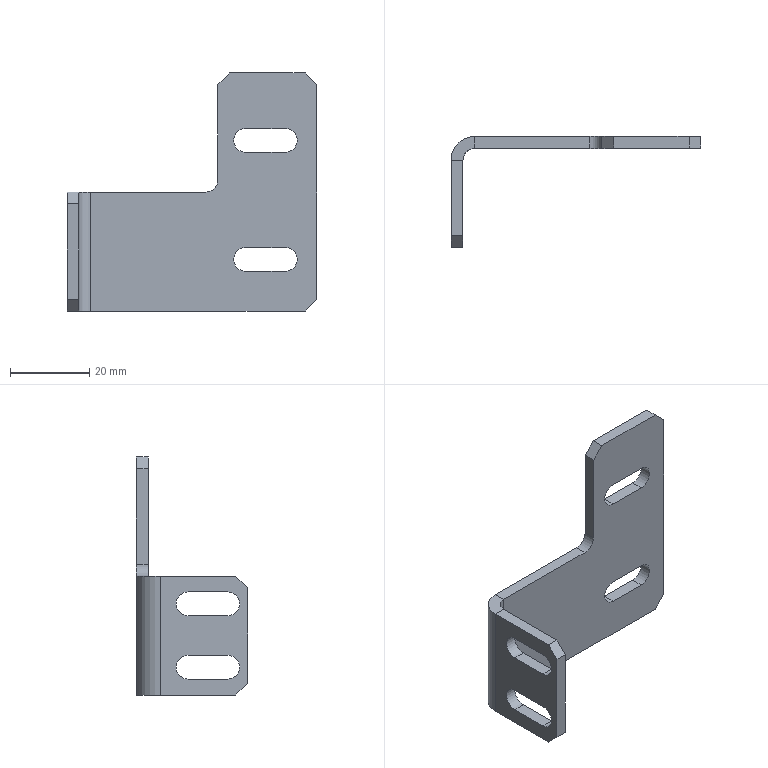Part | NX | features BREP 1 | 1 solid | 38 faces | box 63 x 28 x 60 mm | volume 8875 mm3 | plane 27 | cylinder 11 | commonest cylinder face diameters 6 x10 12 x1
STEP:
#1=CARTESIAN_POINT('',(0.,-3.,30.));
#2=VERTEX_POINT('',#1);
#3=CARTESIAN_POINT('',(-3.,-3.,30.));
#4=VERTEX_POINT('',#3);
#5=CARTESIAN_POINT('',(0.,-3.,30.));
#6=DIRECTION('',(-1.,0.,0.));
#7=VECTOR('',#6,1000.);
#8=LINE('',#5,#7);
#9=EDGE_CURVE('',#2,#4,#8,.T.);
#10=ORIENTED_EDGE('',*,*,#9,.F.);
#11=CARTESIAN_POINT('',(3.,0.,30.));
#12=VERTEX_POINT('',#11);
#13=CARTESIAN_POINT('',(3.,-3.,30.));
#14=DIRECTION('',(0.,0.,-1.));
#15=DIRECTION('',(1.,0.,0.));
#16=AXIS2_PLACEMENT_3D('',#13,#14,#15);
#17=CIRCLE('',#16,3.);
#18=EDGE_CURVE('',#2,#12,#17,.T.);
#19=ORIENTED_EDGE('',*,*,#18,.T.);
#20=CARTESIAN_POINT('',(3.,3.,30.));
#21=VERTEX_POINT('',#20);
#22=CARTESIAN_POINT('',(3.,3.,30.));
#23=DIRECTION('',(0.,-1.,0.));
#24=VECTOR('',#23,1000.);
#25=LINE('',#22,#24);
#26=EDGE_CURVE('',#21,#12,#25,.T.);
#27=ORIENTED_EDGE('',*,*,#26,.F.);
#28=CARTESIAN_POINT('',(3.,-3.,30.));
#29=DIRECTION('',(0.,0.,-1.));
#30=DIRECTION('',(1.,0.,0.));
#31=AXIS2_PLACEMENT_3D('',#28,#29,#30);
#32=CIRCLE('',#31,6.);
#33=EDGE_CURVE('',#4,#21,#32,.T.);
#34=ORIENTED_EDGE('',*,*,#33,.F.);
#35=EDGE_LOOP('',(#10,#19,#27,#34));
#36=FACE_BOUND('',#35,.T.);
#37=CARTESIAN_POINT('',(0.,-3.,30.));
#38=DIRECTION('',(0.,0.,1.));
#39=DIRECTION('',(-1.,0.,0.));
#40=AXIS2_PLACEMENT_3D('',#37,#38,#39);
#41=PLANE('',#40);
#42=ADVANCED_FACE('',(#36),#41,.T.);
#43=CARTESIAN_POINT('',(-3.,-22.,30.));
#44=VERTEX_POINT('',#43);
#45=CARTESIAN_POINT('',(-3.,-25.,30.));
#46=DIRECTION('',(0.,1.,0.));
#47=VECTOR('',#46,1000.);
#48=LINE('',#45,#47);
#49=EDGE_CURVE('',#44,#4,#48,.T.);
#50=ORIENTED_EDGE('',*,*,#49,.F.);
#51=CARTESIAN_POINT('',(0.,-22.,30.));
#52=VERTEX_POINT('',#51);
#53=CARTESIAN_POINT('',(3.,-22.,30.));
#54=DIRECTION('',(1.,0.,0.));
#55=VECTOR('',#54,1000.);
#56=LINE('',#53,#55);
#57=EDGE_CURVE('',#44,#52,#56,.T.);
#58=ORIENTED_EDGE('',*,*,#57,.T.);
#59=CARTESIAN_POINT('',(0.,-25.,30.));
#60=DIRECTION('',(0.,1.,0.));
#61=VECTOR('',#60,1000.);
#62=LINE('',#59,#61);
#63=EDGE_CURVE('',#52,#2,#62,.T.);
#64=ORIENTED_EDGE('',*,*,#63,.T.);
#65=ORIENTED_EDGE('',*,*,#9,.T.);
#66=EDGE_LOOP('',(#50,#58,#64,#65));
#67=FACE_BOUND('',#66,.T.);
#68=CARTESIAN_POINT('',(3.,3.,30.));
#69=DIRECTION('',(0.,0.,1.));
#70=DIRECTION('',(-1.,0.,0.));
#71=AXIS2_PLACEMENT_3D('',#68,#69,#70);
#72=PLANE('',#71);
#73=ADVANCED_FACE('',(#67),#72,.T.);
#74=CARTESIAN_POINT('',(3.,0.,0.));
#75=VERTEX_POINT('',#74);
#76=CARTESIAN_POINT('',(3.,3.,0.));
#77=VERTEX_POINT('',#76);
#78=CARTESIAN_POINT('',(3.,0.,0.));
#79=DIRECTION('',(0.,1.,0.));
#80=VECTOR('',#79,1000.);
#81=LINE('',#78,#80);
#82=EDGE_CURVE('',#75,#77,#81,.T.);
#83=ORIENTED_EDGE('',*,*,#82,.F.);
#84=CARTESIAN_POINT('',(0.,-3.,0.));
#85=VERTEX_POINT('',#84);
#86=CARTESIAN_POINT('',(3.,-3.,0.));
#87=DIRECTION('',(0.,0.,-1.));
#88=DIRECTION('',(1.,0.,0.));
#89=AXIS2_PLACEMENT_3D('',#86,#87,#88);
#90=CIRCLE('',#89,3.);
#91=EDGE_CURVE('',#85,#75,#90,.T.);
#92=ORIENTED_EDGE('',*,*,#91,.F.);
#93=CARTESIAN_POINT('',(-3.,-3.,0.));
#94=VERTEX_POINT('',#93);
#95=CARTESIAN_POINT('',(-3.,-3.,0.));
#96=DIRECTION('',(1.,0.,0.));
#97=VECTOR('',#96,1000.);
#98=LINE('',#95,#97);
#99=EDGE_CURVE('',#94,#85,#98,.T.);
#100=ORIENTED_EDGE('',*,*,#99,.F.);
#101=CARTESIAN_POINT('',(3.,-3.,0.));
#102=DIRECTION('',(0.,0.,-1.));
#103=DIRECTION('',(1.,0.,0.));
#104=AXIS2_PLACEMENT_3D('',#101,#102,#103);
#105=CIRCLE('',#104,6.);
#106=EDGE_CURVE('',#94,#77,#105,.T.);
#107=ORIENTED_EDGE('',*,*,#106,.T.);
#108=EDGE_LOOP('',(#83,#92,#100,#107));
#109=FACE_BOUND('',#108,.T.);
#110=CARTESIAN_POINT('',(3.,0.,0.));
#111=DIRECTION('',(0.,0.,-1.));
#112=DIRECTION('',(1.,0.,0.));
#113=AXIS2_PLACEMENT_3D('',#110,#111,#112);
#114=PLANE('',#113);
#115=ADVANCED_FACE('',(#109),#114,.T.);
#116=CARTESIAN_POINT('',(57.,3.,0.));
#117=VERTEX_POINT('',#116);
#118=CARTESIAN_POINT('',(0.,3.,0.));
#119=DIRECTION('',(1.,0.,0.));
#120=VECTOR('',#119,1000.);
#121=LINE('',#118,#120);
#122=EDGE_CURVE('',#77,#117,#121,.T.);
#123=ORIENTED_EDGE('',*,*,#122,.T.);
#124=CARTESIAN_POINT('',(57.,0.,0.));
#125=VERTEX_POINT('',#124);
#126=CARTESIAN_POINT('',(57.,-3.,0.));
#127=DIRECTION('',(0.,-1.,0.));
#128=VECTOR('',#127,1000.);
#129=LINE('',#126,#128);
#130=EDGE_CURVE('',#117,#125,#129,.T.);
#131=ORIENTED_EDGE('',*,*,#130,.T.);
#132=CARTESIAN_POINT('',(0.,0.,0.));
#133=DIRECTION('',(1.,0.,0.));
#134=VECTOR('',#133,1000.);
#135=LINE('',#132,#134);
#136=EDGE_CURVE('',#75,#125,#135,.T.);
#137=ORIENTED_EDGE('',*,*,#136,.F.);
#138=ORIENTED_EDGE('',*,*,#82,.T.);
#139=EDGE_LOOP('',(#123,#131,#137,#138));
#140=FACE_BOUND('',#139,.T.);
#141=CARTESIAN_POINT('',(-3.,-3.,0.));
#142=DIRECTION('',(0.,0.,-1.));
#143=DIRECTION('',(1.,0.,0.));
#144=AXIS2_PLACEMENT_3D('',#141,#142,#143);
#145=PLANE('',#144);
#146=ADVANCED_FACE('',(#140),#145,.T.);
#147=CARTESIAN_POINT('',(52.,0.,46.));
#148=VERTEX_POINT('',#147);
#149=CARTESIAN_POINT('',(42.,0.,46.));
#150=VERTEX_POINT('',#149);
#151=CARTESIAN_POINT('',(52.,0.,46.));
#152=DIRECTION('',(-1.,0.,0.));
#153=VECTOR('',#152,1000.);
#154=LINE('',#151,#153);
#155=EDGE_CURVE('',#148,#150,#154,.T.);
#156=ORIENTED_EDGE('',*,*,#155,.F.);
#157=CARTESIAN_POINT('',(52.,0.,40.));
#158=VERTEX_POINT('',#157);
#159=CARTESIAN_POINT('',(52.,0.,43.));
#160=DIRECTION('',(0.,-1.,0.));
#161=DIRECTION('',(0.,0.,1.));
#162=AXIS2_PLACEMENT_3D('',#159,#160,#161);
#163=CIRCLE('',#162,3.);
#164=EDGE_CURVE('',#158,#148,#163,.T.);
#165=ORIENTED_EDGE('',*,*,#164,.F.);
#166=CARTESIAN_POINT('',(42.,0.,40.));
#167=VERTEX_POINT('',#166);
#168=CARTESIAN_POINT('',(52.,0.,40.));
#169=DIRECTION('',(1.,0.,0.));
#170=VECTOR('',#169,1000.);
#171=LINE('',#168,#170);
#172=EDGE_CURVE('',#167,#158,#171,.T.);
#173=ORIENTED_EDGE('',*,*,#172,.F.);
#174=CARTESIAN_POINT('',(42.,0.,43.));
#175=DIRECTION('',(0.,-1.,0.));
#176=DIRECTION('',(0.,0.,1.));
#177=AXIS2_PLACEMENT_3D('',#174,#175,#176);
#178=CIRCLE('',#177,3.);
#179=EDGE_CURVE('',#150,#167,#178,.T.);
#180=ORIENTED_EDGE('',*,*,#179,.F.);
#181=EDGE_LOOP('',(#156,#165,#173,#180));
#182=FACE_BOUND('',#181,.T.);
#183=CARTESIAN_POINT('',(52.,0.,16.));
#184=VERTEX_POINT('',#183);
#185=CARTESIAN_POINT('',(42.,0.,16.));
#186=VERTEX_POINT('',#185);
#187=CARTESIAN_POINT('',(52.,0.,16.));
#188=DIRECTION('',(-1.,0.,0.));
#189=VECTOR('',#188,1000.);
#190=LINE('',#187,#189);
#191=EDGE_CURVE('',#184,#186,#190,.T.);
#192=ORIENTED_EDGE('',*,*,#191,.F.);
#193=CARTESIAN_POINT('',(52.,0.,10.));
#194=VERTEX_POINT('',#193);
#195=CARTESIAN_POINT('',(52.,0.,13.));
#196=DIRECTION('',(0.,-1.,0.));
#197=DIRECTION('',(0.,0.,1.));
#198=AXIS2_PLACEMENT_3D('',#195,#196,#197);
#199=CIRCLE('',#198,3.);
#200=EDGE_CURVE('',#194,#184,#199,.T.);
#201=ORIENTED_EDGE('',*,*,#200,.F.);
#202=CARTESIAN_POINT('',(42.,0.,10.));
#203=VERTEX_POINT('',#202);
#204=CARTESIAN_POINT('',(52.,0.,10.));
#205=DIRECTION('',(1.,0.,0.));
#206=VECTOR('',#205,1000.);
#207=LINE('',#204,#206);
#208=EDGE_CURVE('',#203,#194,#207,.T.);
#209=ORIENTED_EDGE('',*,*,#208,.F.);
#210=CARTESIAN_POINT('',(42.,0.,13.));
#211=DIRECTION('',(0.,-1.,0.));
#212=DIRECTION('',(0.,0.,1.));
#213=AXIS2_PLACEMENT_3D('',#210,#211,#212);
#214=CIRCLE('',#213,3.);
#215=EDGE_CURVE('',#186,#203,#214,.T.);
#216=ORIENTED_EDGE('',*,*,#215,.F.);
#217=EDGE_LOOP('',(#192,#201,#209,#216));
#218=FACE_BOUND('',#217,.T.);
#219=CARTESIAN_POINT('',(57.,0.,60.));
#220=VERTEX_POINT('',#219);
#221=CARTESIAN_POINT('',(38.,0.,60.));
#222=VERTEX_POINT('',#221);
#223=CARTESIAN_POINT('',(60.,0.,60.));
#224=DIRECTION('',(-1.,0.,0.));
#225=VECTOR('',#224,1000.);
#226=LINE('',#223,#225);
#227=EDGE_CURVE('',#220,#222,#226,.T.);
#228=ORIENTED_EDGE('',*,*,#227,.T.);
#229=CARTESIAN_POINT('',(35.,0.,57.));
#230=VERTEX_POINT('',#229);
#231=CARTESIAN_POINT('',(38.,0.,60.));
#232=DIRECTION('',(-0.7071,0.,-0.7071));
#233=VECTOR('',#232,1000.);
#234=LINE('',#231,#233);
#235=EDGE_CURVE('',#222,#230,#234,.T.);
#236=ORIENTED_EDGE('',*,*,#235,.T.);
#237=CARTESIAN_POINT('',(35.,0.,33.));
#238=VERTEX_POINT('',#237);
#239=CARTESIAN_POINT('',(35.,0.,30.));
#240=DIRECTION('',(0.,0.,-1.));
#241=VECTOR('',#240,1000.);
#242=LINE('',#239,#241);
#243=EDGE_CURVE('',#230,#238,#242,.T.);
#244=ORIENTED_EDGE('',*,*,#243,.T.);
#245=CARTESIAN_POINT('',(32.,0.,30.));
#246=VERTEX_POINT('',#245);
#247=CARTESIAN_POINT('',(32.,0.,33.));
#248=DIRECTION('',(0.,1.,0.));
#249=DIRECTION('',(0.,0.,1.));
#250=AXIS2_PLACEMENT_3D('',#247,#248,#249);
#251=CIRCLE('',#250,3.);
#252=EDGE_CURVE('',#238,#246,#251,.T.);
#253=ORIENTED_EDGE('',*,*,#252,.T.);
#254=CARTESIAN_POINT('',(0.,0.,30.));
#255=DIRECTION('',(1.,0.,0.));
#256=VECTOR('',#255,1000.);
#257=LINE('',#254,#256);
#258=EDGE_CURVE('',#12,#246,#257,.T.);
#259=ORIENTED_EDGE('',*,*,#258,.F.);
#260=CARTESIAN_POINT('',(3.,0.,30.));
#261=DIRECTION('',(0.,0.,-1.));
#262=VECTOR('',#261,1000.);
#263=LINE('',#260,#262);
#264=EDGE_CURVE('',#12,#75,#263,.T.);
#265=ORIENTED_EDGE('',*,*,#264,.T.);
#266=ORIENTED_EDGE('',*,*,#136,.T.);
#267=CARTESIAN_POINT('',(60.,0.,3.));
#268=VERTEX_POINT('',#267);
#269=CARTESIAN_POINT('',(57.,0.,0.));
#270=DIRECTION('',(0.7071,0.,0.7071));
#271=VECTOR('',#270,1000.);
#272=LINE('',#269,#271);
#273=EDGE_CURVE('',#125,#268,#272,.T.);
#274=ORIENTED_EDGE('',*,*,#273,.T.);
#275=CARTESIAN_POINT('',(60.,0.,57.));
#276=VERTEX_POINT('',#275);
#277=CARTESIAN_POINT('',(60.,0.,30.));
#278=DIRECTION('',(0.,0.,-1.));
#279=VECTOR('',#278,1000.);
#280=LINE('',#277,#279);
#281=EDGE_CURVE('',#276,#268,#280,.T.);
#282=ORIENTED_EDGE('',*,*,#281,.F.);
#283=CARTESIAN_POINT('',(60.,0.,57.));
#284=DIRECTION('',(-0.7071,0.,0.7071));
#285=VECTOR('',#284,1000.);
#286=LINE('',#283,#285);
#287=EDGE_CURVE('',#276,#220,#286,.T.);
#288=ORIENTED_EDGE('',*,*,#287,.T.);
#289=EDGE_LOOP('',(#228,#236,#244,#253,#259,#265,#266,#274,#282,#288));
#290=FACE_BOUND('',#289,.T.);
#291=CARTESIAN_POINT('',(0.,0.,30.));
#292=DIRECTION('',(0.,1.,0.));
#293=DIRECTION('',(0.,0.,-1.));
#294=AXIS2_PLACEMENT_3D('',#291,#292,#293);
#295=PLANE('',#294);
#296=ADVANCED_FACE('',(#182,#218,#290),#295,.F.);
#297=CARTESIAN_POINT('',(60.,3.,57.));
#298=VERTEX_POINT('',#297);
#299=CARTESIAN_POINT('',(60.,3.,3.));
#300=VERTEX_POINT('',#299);
#301=CARTESIAN_POINT('',(60.,3.,30.));
#302=DIRECTION('',(0.,0.,-1.));
#303=VECTOR('',#302,1000.);
#304=LINE('',#301,#303);
#305=EDGE_CURVE('',#298,#300,#304,.T.);
#306=ORIENTED_EDGE('',*,*,#305,.F.);
#307=CARTESIAN_POINT('',(60.,3.,57.));
#308=DIRECTION('',(0.,-1.,0.));
#309=VECTOR('',#308,1000.);
#310=LINE('',#307,#309);
#311=EDGE_CURVE('',#298,#276,#310,.T.);
#312=ORIENTED_EDGE('',*,*,#311,.T.);
#313=ORIENTED_EDGE('',*,*,#281,.T.);
#314=CARTESIAN_POINT('',(60.,3.,3.));
#315=DIRECTION('',(0.,1.,0.));
#316=VECTOR('',#315,1000.);
#317=LINE('',#314,#316);
#318=EDGE_CURVE('',#268,#300,#317,.T.);
#319=ORIENTED_EDGE('',*,*,#318,.T.);
#320=EDGE_LOOP('',(#306,#312,#313,#319));
#321=FACE_BOUND('',#320,.T.);
#322=CARTESIAN_POINT('',(60.,3.,30.));
#323=DIRECTION('',(1.,0.,0.));
#324=DIRECTION('',(0.,0.,1.));
#325=AXIS2_PLACEMENT_3D('',#322,#323,#324);
#326=PLANE('',#325);
#327=ADVANCED_FACE('',(#321),#326,.T.);
#328=CARTESIAN_POINT('',(52.,3.,46.));
#329=VERTEX_POINT('',#328);
#330=CARTESIAN_POINT('',(52.,3.,40.));
#331=VERTEX_POINT('',#330);
#332=CARTESIAN_POINT('',(52.,3.,43.));
#333=DIRECTION('',(0.,1.,0.));
#334=DIRECTION('',(0.,0.,1.));
#335=AXIS2_PLACEMENT_3D('',#332,#333,#334);
#336=CIRCLE('',#335,3.);
#337=EDGE_CURVE('',#329,#331,#336,.T.);
#338=ORIENTED_EDGE('',*,*,#337,.F.);
#339=CARTESIAN_POINT('',(42.,3.,46.));
#340=VERTEX_POINT('',#339);
#341=CARTESIAN_POINT('',(52.,3.,46.));
#342=DIRECTION('',(1.,0.,0.));
#343=VECTOR('',#342,1000.);
#344=LINE('',#341,#343);
#345=EDGE_CURVE('',#340,#329,#344,.T.);
#346=ORIENTED_EDGE('',*,*,#345,.F.);
#347=CARTESIAN_POINT('',(42.,3.,40.));
#348=VERTEX_POINT('',#347);
#349=CARTESIAN_POINT('',(42.,3.,43.));
#350=DIRECTION('',(0.,1.,0.));
#351=DIRECTION('',(0.,0.,1.));
#352=AXIS2_PLACEMENT_3D('',#349,#350,#351);
#353=CIRCLE('',#352,3.);
#354=EDGE_CURVE('',#348,#340,#353,.T.);
#355=ORIENTED_EDGE('',*,*,#354,.F.);
#356=CARTESIAN_POINT('',(52.,3.,40.));
#357=DIRECTION('',(-1.,0.,0.));
#358=VECTOR('',#357,1000.);
#359=LINE('',#356,#358);
#360=EDGE_CURVE('',#331,#348,#359,.T.);
#361=ORIENTED_EDGE('',*,*,#360,.F.);
#362=EDGE_LOOP('',(#338,#346,#355,#361));
#363=FACE_BOUND('',#362,.T.);
#364=CARTESIAN_POINT('',(52.,3.,16.));
#365=VERTEX_POINT('',#364);
#366=CARTESIAN_POINT('',(52.,3.,10.));
#367=VERTEX_POINT('',#366);
#368=CARTESIAN_POINT('',(52.,3.,13.));
#369=DIRECTION('',(0.,1.,0.));
#370=DIRECTION('',(0.,0.,1.));
#371=AXIS2_PLACEMENT_3D('',#368,#369,#370);
#372=CIRCLE('',#371,3.);
#373=EDGE_CURVE('',#365,#367,#372,.T.);
#374=ORIENTED_EDGE('',*,*,#373,.F.);
#375=CARTESIAN_POINT('',(42.,3.,16.));
#376=VERTEX_POINT('',#375);
#377=CARTESIAN_POINT('',(52.,3.,16.));
#378=DIRECTION('',(1.,0.,0.));
#379=VECTOR('',#378,1000.);
#380=LINE('',#377,#379);
#381=EDGE_CURVE('',#376,#365,#380,.T.);
#382=ORIENTED_EDGE('',*,*,#381,.F.);
#383=CARTESIAN_POINT('',(42.,3.,10.));
#384=VERTEX_POINT('',#383);
#385=CARTESIAN_POINT('',(42.,3.,13.));
#386=DIRECTION('',(0.,1.,0.));
#387=DIRECTION('',(0.,0.,1.));
#388=AXIS2_PLACEMENT_3D('',#385,#386,#387);
#389=CIRCLE('',#388,3.);
#390=EDGE_CURVE('',#384,#376,#389,.T.);
#391=ORIENTED_EDGE('',*,*,#390,.F.);
#392=CARTESIAN_POINT('',(52.,3.,10.));
#393=DIRECTION('',(-1.,0.,0.));
#394=VECTOR('',#393,1000.);
#395=LINE('',#392,#394);
#396=EDGE_CURVE('',#367,#384,#395,.T.);
#397=ORIENTED_EDGE('',*,*,#396,.F.);
#398=EDGE_LOOP('',(#374,#382,#391,#397));
#399=FACE_BOUND('',#398,.T.);
#400=CARTESIAN_POINT('',(35.,3.,57.));
#401=VERTEX_POINT('',#400);
#402=CARTESIAN_POINT('',(35.,3.,33.));
#403=VERTEX_POINT('',#402);
#404=CARTESIAN_POINT('',(35.,3.,30.));
#405=DIRECTION('',(0.,0.,-1.));
#406=VECTOR('',#405,1000.);
#407=LINE('',#404,#406);
#408=EDGE_CURVE('',#401,#403,#407,.T.);
#409=ORIENTED_EDGE('',*,*,#408,.F.);
#410=CARTESIAN_POINT('',(38.,3.,60.));
#411=VERTEX_POINT('',#410);
#412=CARTESIAN_POINT('',(4.,3.,26.));
#413=DIRECTION('',(0.7071,0.,0.7071));
#414=VECTOR('',#413,1000.);
#415=LINE('',#412,#414);
#416=EDGE_CURVE('',#401,#411,#415,.T.);
#417=ORIENTED_EDGE('',*,*,#416,.T.);
#418=CARTESIAN_POINT('',(57.,3.,60.));
#419=VERTEX_POINT('',#418);
#420=CARTESIAN_POINT('',(60.,3.,60.));
#421=DIRECTION('',(-1.,0.,0.));
#422=VECTOR('',#421,1000.);
#423=LINE('',#420,#422);
#424=EDGE_CURVE('',#419,#411,#423,.T.);
#425=ORIENTED_EDGE('',*,*,#424,.F.);
#426=CARTESIAN_POINT('',(43.5,3.,73.5));
#427=DIRECTION('',(0.7071,0.,-0.7071));
#428=VECTOR('',#427,1000.);
#429=LINE('',#426,#428);
#430=EDGE_CURVE('',#419,#298,#429,.T.);
#431=ORIENTED_EDGE('',*,*,#430,.T.);
#432=ORIENTED_EDGE('',*,*,#305,.T.);
#433=CARTESIAN_POINT('',(43.5,3.,-13.5));
#434=DIRECTION('',(-0.7071,0.,-0.7071));
#435=VECTOR('',#434,1000.);
#436=LINE('',#433,#435);
#437=EDGE_CURVE('',#300,#117,#436,.T.);
#438=ORIENTED_EDGE('',*,*,#437,.T.);
#439=ORIENTED_EDGE('',*,*,#122,.F.);
#440=CARTESIAN_POINT('',(3.,3.,30.));
#441=DIRECTION('',(0.,0.,-1.));
#442=VECTOR('',#441,1000.);
#443=LINE('',#440,#442);
#444=EDGE_CURVE('',#21,#77,#443,.T.);
#445=ORIENTED_EDGE('',*,*,#444,.F.);
#446=CARTESIAN_POINT('',(32.,3.,30.));
#447=VERTEX_POINT('',#446);
#448=CARTESIAN_POINT('',(0.,3.,30.));
#449=DIRECTION('',(1.,0.,0.));
#450=VECTOR('',#449,1000.);
#451=LINE('',#448,#450);
#452=EDGE_CURVE('',#21,#447,#451,.T.);
#453=ORIENTED_EDGE('',*,*,#452,.T.);
#454=CARTESIAN_POINT('',(32.,3.,33.));
#455=DIRECTION('',(0.,-1.,0.));
#456=DIRECTION('',(0.,0.,1.));
#457=AXIS2_PLACEMENT_3D('',#454,#455,#456);
#458=CIRCLE('',#457,3.);
#459=EDGE_CURVE('',#447,#403,#458,.T.);
#460=ORIENTED_EDGE('',*,*,#459,.T.);
#461=EDGE_LOOP('',(#409,#417,#425,#431,#432,#438,#439,#445,#453,#460));
#462=FACE_BOUND('',#461,.T.);
#463=CARTESIAN_POINT('',(0.,3.,30.));
#464=DIRECTION('',(0.,1.,0.));
#465=DIRECTION('',(0.,0.,-1.));
#466=AXIS2_PLACEMENT_3D('',#463,#464,#465);
#467=PLANE('',#466);
#468=ADVANCED_FACE('',(#363,#399,#462),#467,.T.);
#469=ORIENTED_EDGE('',*,*,#106,.F.);
#470=CARTESIAN_POINT('',(-3.,-3.,30.));
#471=DIRECTION('',(0.,0.,-1.));
#472=VECTOR('',#471,1000.);
#473=LINE('',#470,#472);
#474=EDGE_CURVE('',#4,#94,#473,.T.);
#475=ORIENTED_EDGE('',*,*,#474,.F.);
#476=ORIENTED_EDGE('',*,*,#33,.T.);
#477=ORIENTED_EDGE('',*,*,#444,.T.);
#478=EDGE_LOOP('',(#469,#475,#476,#477));
#479=FACE_BOUND('',#478,.T.);
#480=CARTESIAN_POINT('',(3.,-3.,30.));
#481=DIRECTION('',(0.,0.,-1.));
#482=DIRECTION('',(1.,0.,0.));
#483=AXIS2_PLACEMENT_3D('',#480,#481,#482);
#484=CYLINDRICAL_SURFACE('',#483,6.);
#485=ADVANCED_FACE('',(#479),#484,.T.);
#486=CARTESIAN_POINT('',(-3.,-10.,26.));
#487=VERTEX_POINT('',#486);
#488=CARTESIAN_POINT('',(-3.,-20.,26.));
#489=VERTEX_POINT('',#488);
#490=CARTESIAN_POINT('',(-3.,-10.,26.));
#491=DIRECTION('',(0.,-1.,0.));
#492=VECTOR('',#491,1000.);
#493=LINE('',#490,#492);
#494=EDGE_CURVE('',#487,#489,#493,.T.);
#495=ORIENTED_EDGE('',*,*,#494,.T.);
#496=CARTESIAN_POINT('',(-3.,-20.,20.));
#497=VERTEX_POINT('',#496);
#498=CARTESIAN_POINT('',(-3.,-20.,23.));
#499=DIRECTION('',(1.,0.,0.));
#500=DIRECTION('',(0.,0.,1.));
#501=AXIS2_PLACEMENT_3D('',#498,#499,#500);
#502=CIRCLE('',#501,3.);
#503=EDGE_CURVE('',#489,#497,#502,.T.);
#504=ORIENTED_EDGE('',*,*,#503,.T.);
#505=CARTESIAN_POINT('',(-3.,-10.,20.));
#506=VERTEX_POINT('',#505);
#507=CARTESIAN_POINT('',(-3.,-10.,20.));
#508=DIRECTION('',(0.,1.,0.));
#509=VECTOR('',#508,1000.);
#510=LINE('',#507,#509);
#511=EDGE_CURVE('',#497,#506,#510,.T.);
#512=ORIENTED_EDGE('',*,*,#511,.T.);
#513=CARTESIAN_POINT('',(-3.,-10.,23.));
#514=DIRECTION('',(1.,0.,0.));
#515=DIRECTION('',(0.,0.,1.));
#516=AXIS2_PLACEMENT_3D('',#513,#514,#515);
#517=CIRCLE('',#516,3.);
#518=EDGE_CURVE('',#506,#487,#517,.T.);
#519=ORIENTED_EDGE('',*,*,#518,.T.);
#520=EDGE_LOOP('',(#495,#504,#512,#519));
#521=FACE_BOUND('',#520,.T.);
#522=CARTESIAN_POINT('',(-3.,-10.,10.));
#523=VERTEX_POINT('',#522);
#524=CARTESIAN_POINT('',(-3.,-20.,10.));
#525=VERTEX_POINT('',#524);
#526=CARTESIAN_POINT('',(-3.,-10.,10.));
#527=DIRECTION('',(0.,-1.,0.));
#528=VECTOR('',#527,1000.);
#529=LINE('',#526,#528);
#530=EDGE_CURVE('',#523,#525,#529,.T.);
#531=ORIENTED_EDGE('',*,*,#530,.T.);
#532=CARTESIAN_POINT('',(-3.,-20.,4.));
#533=VERTEX_POINT('',#532);
#534=CARTESIAN_POINT('',(-3.,-20.,7.));
#535=DIRECTION('',(1.,0.,0.));
#536=DIRECTION('',(0.,0.,1.));
#537=AXIS2_PLACEMENT_3D('',#534,#535,#536);
#538=CIRCLE('',#537,3.);
#539=EDGE_CURVE('',#525,#533,#538,.T.);
#540=ORIENTED_EDGE('',*,*,#539,.T.);
#541=CARTESIAN_POINT('',(-3.,-10.,4.));
#542=VERTEX_POINT('',#541);
#543=CARTESIAN_POINT('',(-3.,-10.,4.));
#544=DIRECTION('',(0.,1.,0.));
#545=VECTOR('',#544,1000.);
#546=LINE('',#543,#545);
#547=EDGE_CURVE('',#533,#542,#546,.T.);
#548=ORIENTED_EDGE('',*,*,#547,.T.);
#549=CARTESIAN_POINT('',(-3.,-10.,7.));
#550=DIRECTION('',(1.,0.,0.));
#551=DIRECTION('',(0.,0.,1.));
#552=AXIS2_PLACEMENT_3D('',#549,#550,#551);
#553=CIRCLE('',#552,3.);
#554=EDGE_CURVE('',#542,#523,#553,.T.);
#555=ORIENTED_EDGE('',*,*,#554,.T.);
#556=EDGE_LOOP('',(#531,#540,#548,#555));
#557=FACE_BOUND('',#556,.T.);
#558=CARTESIAN_POINT('',(-3.,-25.,27.));
#559=VERTEX_POINT('',#558);
#560=CARTESIAN_POINT('',(-3.,-25.,3.));
#561=VERTEX_POINT('',#560);
#562=CARTESIAN_POINT('',(-3.,-25.,30.));
#563=DIRECTION('',(0.,0.,-1.));
#564=VECTOR('',#563,1000.);
#565=LINE('',#562,#564);
#566=EDGE_CURVE('',#559,#561,#565,.T.);
#567=ORIENTED_EDGE('',*,*,#566,.F.);
#568=CARTESIAN_POINT('',(-3.,-23.5,28.5));
#569=DIRECTION('',(0.,0.7071,0.7071));
#570=VECTOR('',#569,1000.);
#571=LINE('',#568,#570);
#572=EDGE_CURVE('',#559,#44,#571,.T.);
#573=ORIENTED_EDGE('',*,*,#572,.T.);
#574=ORIENTED_EDGE('',*,*,#49,.T.);
#575=ORIENTED_EDGE('',*,*,#474,.T.);
#576=CARTESIAN_POINT('',(-3.,-22.,0.));
#577=VERTEX_POINT('',#576);
#578=CARTESIAN_POINT('',(-3.,-25.,0.));
#579=DIRECTION('',(0.,1.,0.));
#580=VECTOR('',#579,1000.);
#581=LINE('',#578,#580);
#582=EDGE_CURVE('',#577,#94,#581,.T.);
#583=ORIENTED_EDGE('',*,*,#582,.F.);
#584=CARTESIAN_POINT('',(-3.,-38.5,16.5));
#585=DIRECTION('',(0.,-0.7071,0.7071));
#586=VECTOR('',#585,1000.);
#587=LINE('',#584,#586);
#588=EDGE_CURVE('',#577,#561,#587,.T.);
#589=ORIENTED_EDGE('',*,*,#588,.T.);
#590=EDGE_LOOP('',(#567,#573,#574,#575,#583,#589));
#591=FACE_BOUND('',#590,.T.);
#592=CARTESIAN_POINT('',(-3.,-25.,30.));
#593=DIRECTION('',(-1.,0.,0.));
#594=DIRECTION('',(0.,0.,-1.));
#595=AXIS2_PLACEMENT_3D('',#592,#593,#594);
#596=PLANE('',#595);
#597=ADVANCED_FACE('',(#521,#557,#591),#596,.T.);
#598=CARTESIAN_POINT('',(0.,-25.,27.));
#599=VERTEX_POINT('',#598);
#600=CARTESIAN_POINT('',(0.,-25.,3.));
#601=VERTEX_POINT('',#600);
#602=CARTESIAN_POINT('',(0.,-25.,30.));
#603=DIRECTION('',(0.,0.,-1.));
#604=VECTOR('',#603,1000.);
#605=LINE('',#602,#604);
#606=EDGE_CURVE('',#599,#601,#605,.T.);
#607=ORIENTED_EDGE('',*,*,#606,.F.);
#608=CARTESIAN_POINT('',(0.,-25.,27.));
#609=DIRECTION('',(-1.,0.,0.));
#610=VECTOR('',#609,1000.);
#611=LINE('',#608,#610);
#612=EDGE_CURVE('',#599,#559,#611,.T.);
#613=ORIENTED_EDGE('',*,*,#612,.T.);
#614=ORIENTED_EDGE('',*,*,#566,.T.);
#615=CARTESIAN_POINT('',(0.,-25.,3.));
#616=DIRECTION('',(1.,0.,0.));
#617=VECTOR('',#616,1000.);
#618=LINE('',#615,#617);
#619=EDGE_CURVE('',#561,#601,#618,.T.);
#620=ORIENTED_EDGE('',*,*,#619,.T.);
#621=EDGE_LOOP('',(#607,#613,#614,#620));
#622=FACE_BOUND('',#621,.T.);
#623=CARTESIAN_POINT('',(0.,-25.,30.));
#624=DIRECTION('',(0.,-1.,0.));
#625=DIRECTION('',(0.,0.,1.));
#626=AXIS2_PLACEMENT_3D('',#623,#624,#625);
#627=PLANE('',#626);
#628=ADVANCED_FACE('',(#622),#627,.T.);
#629=CARTESIAN_POINT('',(0.,-20.,26.));
#630=VERTEX_POINT('',#629);
#631=CARTESIAN_POINT('',(0.,-20.,20.));
#632=VERTEX_POINT('',#631);
#633=CARTESIAN_POINT('',(0.,-20.,23.));
#634=DIRECTION('',(1.,0.,0.));
#635=DIRECTION('',(0.,0.,-1.));
#636=AXIS2_PLACEMENT_3D('',#633,#634,#635);
#637=CIRCLE('',#636,3.);
#638=EDGE_CURVE('',#630,#632,#637,.T.);
#639=ORIENTED_EDGE('',*,*,#638,.F.);
#640=CARTESIAN_POINT('',(0.,-10.,26.));
#641=VERTEX_POINT('',#640);
#642=CARTESIAN_POINT('',(0.,-10.,26.));
#643=DIRECTION('',(0.,-1.,0.));
#644=VECTOR('',#643,1000.);
#645=LINE('',#642,#644);
#646=EDGE_CURVE('',#641,#630,#645,.T.);
#647=ORIENTED_EDGE('',*,*,#646,.F.);
#648=CARTESIAN_POINT('',(0.,-10.,20.));
#649=VERTEX_POINT('',#648);
#650=CARTESIAN_POINT('',(0.,-10.,23.));
#651=DIRECTION('',(1.,0.,0.));
#652=DIRECTION('',(0.,0.,-1.));
#653=AXIS2_PLACEMENT_3D('',#650,#651,#652);
#654=CIRCLE('',#653,3.);
#655=EDGE_CURVE('',#649,#641,#654,.T.);
#656=ORIENTED_EDGE('',*,*,#655,.F.);
#657=CARTESIAN_POINT('',(0.,-10.,20.));
#658=DIRECTION('',(0.,1.,0.));
#659=VECTOR('',#658,1000.);
#660=LINE('',#657,#659);
#661=EDGE_CURVE('',#632,#649,#660,.T.);
#662=ORIENTED_EDGE('',*,*,#661,.F.);
#663=EDGE_LOOP('',(#639,#647,#656,#662));
#664=FACE_BOUND('',#663,.T.);
#665=CARTESIAN_POINT('',(0.,-20.,10.));
#666=VERTEX_POINT('',#665);
#667=CARTESIAN_POINT('',(0.,-20.,4.));
#668=VERTEX_POINT('',#667);
#669=CARTESIAN_POINT('',(0.,-20.,7.));
#670=DIRECTION('',(1.,0.,0.));
#671=DIRECTION('',(0.,0.,-1.));
#672=AXIS2_PLACEMENT_3D('',#669,#670,#671);
#673=CIRCLE('',#672,3.);
#674=EDGE_CURVE('',#666,#668,#673,.T.);
#675=ORIENTED_EDGE('',*,*,#674,.F.);
#676=CARTESIAN_POINT('',(0.,-10.,10.));
#677=VERTEX_POINT('',#676);
#678=CARTESIAN_POINT('',(0.,-10.,10.));
#679=DIRECTION('',(0.,-1.,0.));
#680=VECTOR('',#679,1000.);
#681=LINE('',#678,#680);
#682=EDGE_CURVE('',#677,#666,#681,.T.);
#683=ORIENTED_EDGE('',*,*,#682,.F.);
#684=CARTESIAN_POINT('',(0.,-10.,4.));
#685=VERTEX_POINT('',#684);
#686=CARTESIAN_POINT('',(0.,-10.,7.));
#687=DIRECTION('',(1.,0.,0.));
#688=DIRECTION('',(0.,0.,-1.));
#689=AXIS2_PLACEMENT_3D('',#686,#687,#688);
#690=CIRCLE('',#689,3.);
#691=EDGE_CURVE('',#685,#677,#690,.T.);
#692=ORIENTED_EDGE('',*,*,#691,.F.);
#693=CARTESIAN_POINT('',(0.,-10.,4.));
#694=DIRECTION('',(0.,1.,0.));
#695=VECTOR('',#694,1000.);
#696=LINE('',#693,#695);
#697=EDGE_CURVE('',#668,#685,#696,.T.);
#698=ORIENTED_EDGE('',*,*,#697,.F.);
#699=EDGE_LOOP('',(#675,#683,#692,#698));
#700=FACE_BOUND('',#699,.T.);
#701=ORIENTED_EDGE('',*,*,#63,.F.);
#702=CARTESIAN_POINT('',(0.,-25.,27.));
#703=DIRECTION('',(0.,-0.7071,-0.7071));
#704=VECTOR('',#703,1000.);
#705=LINE('',#702,#704);
#706=EDGE_CURVE('',#52,#599,#705,.T.);
#707=ORIENTED_EDGE('',*,*,#706,.T.);
#708=ORIENTED_EDGE('',*,*,#606,.T.);
#709=CARTESIAN_POINT('',(0.,-22.,0.));
#710=VERTEX_POINT('',#709);
#711=CARTESIAN_POINT('',(0.,-22.,0.));
#712=DIRECTION('',(0.,0.7071,-0.7071));
#713=VECTOR('',#712,1000.);
#714=LINE('',#711,#713);
#715=EDGE_CURVE('',#601,#710,#714,.T.);
#716=ORIENTED_EDGE('',*,*,#715,.T.);
#717=CARTESIAN_POINT('',(0.,-25.,0.));
#718=DIRECTION('',(0.,1.,0.));
#719=VECTOR('',#718,1000.);
#720=LINE('',#717,#719);
#721=EDGE_CURVE('',#710,#85,#720,.T.);
#722=ORIENTED_EDGE('',*,*,#721,.T.);
#723=CARTESIAN_POINT('',(0.,-3.,30.));
#724=DIRECTION('',(0.,0.,-1.));
#725=VECTOR('',#724,1000.);
#726=LINE('',#723,#725);
#727=EDGE_CURVE('',#2,#85,#726,.T.);
#728=ORIENTED_EDGE('',*,*,#727,.F.);
#729=EDGE_LOOP('',(#701,#707,#708,#716,#722,#728));
#730=FACE_BOUND('',#729,.T.);
#731=CARTESIAN_POINT('',(0.,-25.,30.));
#732=DIRECTION('',(-1.,0.,0.));
#733=DIRECTION('',(0.,0.,-1.));
#734=AXIS2_PLACEMENT_3D('',#731,#732,#733);
#735=PLANE('',#734);
#736=ADVANCED_FACE('',(#664,#700,#730),#735,.F.);
#737=ORIENTED_EDGE('',*,*,#91,.T.);
#738=ORIENTED_EDGE('',*,*,#264,.F.);
#739=ORIENTED_EDGE('',*,*,#18,.F.);
#740=ORIENTED_EDGE('',*,*,#727,.T.);
#741=EDGE_LOOP('',(#737,#738,#739,#740));
#742=FACE_BOUND('',#741,.T.);
#743=CARTESIAN_POINT('',(3.,-3.,30.));
#744=DIRECTION('',(0.,0.,-1.));
#745=DIRECTION('',(1.,0.,0.));
#746=AXIS2_PLACEMENT_3D('',#743,#744,#745);
#747=CYLINDRICAL_SURFACE('',#746,3.);
#748=ADVANCED_FACE('',(#742),#747,.F.);
#749=ORIENTED_EDGE('',*,*,#258,.T.);
#750=CARTESIAN_POINT('',(32.,3.,30.));
#751=DIRECTION('',(0.,1.,0.));
#752=VECTOR('',#751,1000.);
#753=LINE('',#750,#752);
#754=EDGE_CURVE('',#246,#447,#753,.T.);
#755=ORIENTED_EDGE('',*,*,#754,.T.);
#756=ORIENTED_EDGE('',*,*,#452,.F.);
#757=ORIENTED_EDGE('',*,*,#26,.T.);
#758=EDGE_LOOP('',(#749,#755,#756,#757));
#759=FACE_BOUND('',#758,.T.);
#760=CARTESIAN_POINT('',(3.,-3.,30.));
#761=DIRECTION('',(0.,0.,1.));
#762=DIRECTION('',(-1.,0.,0.));
#763=AXIS2_PLACEMENT_3D('',#760,#761,#762);
#764=PLANE('',#763);
#765=ADVANCED_FACE('',(#759),#764,.T.);
#766=ORIENTED_EDGE('',*,*,#721,.F.);
#767=CARTESIAN_POINT('',(-3.,-22.,0.));
#768=DIRECTION('',(-1.,0.,0.));
#769=VECTOR('',#768,1000.);
#770=LINE('',#767,#769);
#771=EDGE_CURVE('',#710,#577,#770,.T.);
#772=ORIENTED_EDGE('',*,*,#771,.T.);
#773=ORIENTED_EDGE('',*,*,#582,.T.);
#774=ORIENTED_EDGE('',*,*,#99,.T.);
#775=EDGE_LOOP('',(#766,#772,#773,#774));
#776=FACE_BOUND('',#775,.T.);
#777=CARTESIAN_POINT('',(3.,-3.,0.));
#778=DIRECTION('',(0.,0.,1.));
#779=DIRECTION('',(-1.,0.,0.));
#780=AXIS2_PLACEMENT_3D('',#777,#778,#779);
#781=PLANE('',#780);
#782=ADVANCED_FACE('',(#776),#781,.F.);
#783=CARTESIAN_POINT('',(-20.088,-10.,10.));
#784=DIRECTION('',(1.,0.,0.));
#785=VECTOR('',#784,1000.);
#786=LINE('',#783,#785);
#787=EDGE_CURVE('',#523,#677,#786,.T.);
#788=ORIENTED_EDGE('',*,*,#787,.T.);
#789=ORIENTED_EDGE('',*,*,#682,.T.);
#790=CARTESIAN_POINT('',(-20.088,-20.,10.));
#791=DIRECTION('',(1.,0.,0.));
#792=VECTOR('',#791,1000.);
#793=LINE('',#790,#792);
#794=EDGE_CURVE('',#525,#666,#793,.T.);
#795=ORIENTED_EDGE('',*,*,#794,.F.);
#796=ORIENTED_EDGE('',*,*,#530,.F.);
#797=EDGE_LOOP('',(#788,#789,#795,#796));
#798=FACE_BOUND('',#797,.T.);
#799=CARTESIAN_POINT('',(-20.088,-10.,10.));
#800=DIRECTION('',(0.,0.,1.));
#801=DIRECTION('',(-1.,0.,0.));
#802=AXIS2_PLACEMENT_3D('',#799,#800,#801);
#803=PLANE('',#802);
#804=ADVANCED_FACE('',(#798),#803,.F.);
#805=ORIENTED_EDGE('',*,*,#794,.T.);
#806=ORIENTED_EDGE('',*,*,#674,.T.);
#807=CARTESIAN_POINT('',(-20.088,-20.,4.));
#808=DIRECTION('',(1.,0.,0.));
#809=VECTOR('',#808,1000.);
#810=LINE('',#807,#809);
#811=EDGE_CURVE('',#533,#668,#810,.T.);
#812=ORIENTED_EDGE('',*,*,#811,.F.);
#813=ORIENTED_EDGE('',*,*,#539,.F.);
#814=EDGE_LOOP('',(#805,#806,#812,#813));
#815=FACE_BOUND('',#814,.T.);
#816=CARTESIAN_POINT('',(-20.088,-20.,7.));
#817=DIRECTION('',(1.,0.,0.));
#818=DIRECTION('',(0.,0.,1.));
#819=AXIS2_PLACEMENT_3D('',#816,#817,#818);
#820=CYLINDRICAL_SURFACE('',#819,3.);
#821=ADVANCED_FACE('',(#815),#820,.F.);
#822=ORIENTED_EDGE('',*,*,#811,.T.);
#823=ORIENTED_EDGE('',*,*,#697,.T.);
#824=CARTESIAN_POINT('',(-20.088,-10.,4.));
#825=DIRECTION('',(1.,0.,0.));
#826=VECTOR('',#825,1000.);
#827=LINE('',#824,#826);
#828=EDGE_CURVE('',#542,#685,#827,.T.);
#829=ORIENTED_EDGE('',*,*,#828,.F.);
#830=ORIENTED_EDGE('',*,*,#547,.F.);
#831=EDGE_LOOP('',(#822,#823,#829,#830));
#832=FACE_BOUND('',#831,.T.);
#833=CARTESIAN_POINT('',(-20.088,-10.,4.));
#834=DIRECTION('',(0.,0.,-1.));
#835=DIRECTION('',(1.,0.,0.));
#836=AXIS2_PLACEMENT_3D('',#833,#834,#835);
#837=PLANE('',#836);
#838=ADVANCED_FACE('',(#832),#837,.F.);
#839=ORIENTED_EDGE('',*,*,#828,.T.);
#840=ORIENTED_EDGE('',*,*,#691,.T.);
#841=ORIENTED_EDGE('',*,*,#787,.F.);
#842=ORIENTED_EDGE('',*,*,#554,.F.);
#843=EDGE_LOOP('',(#839,#840,#841,#842));
#844=FACE_BOUND('',#843,.T.);
#845=CARTESIAN_POINT('',(-20.088,-10.,7.));
#846=DIRECTION('',(1.,0.,0.));
#847=DIRECTION('',(0.,0.,1.));
#848=AXIS2_PLACEMENT_3D('',#845,#846,#847);
#849=CYLINDRICAL_SURFACE('',#848,3.);
#850=ADVANCED_FACE('',(#844),#849,.F.);
#851=CARTESIAN_POINT('',(-20.088,-10.,26.));
#852=DIRECTION('',(1.,0.,0.));
#853=VECTOR('',#852,1000.);
#854=LINE('',#851,#853);
#855=EDGE_CURVE('',#487,#641,#854,.T.);
#856=ORIENTED_EDGE('',*,*,#855,.T.);
#857=ORIENTED_EDGE('',*,*,#646,.T.);
#858=CARTESIAN_POINT('',(-20.088,-20.,26.));
#859=DIRECTION('',(1.,0.,0.));
#860=VECTOR('',#859,1000.);
#861=LINE('',#858,#860);
#862=EDGE_CURVE('',#489,#630,#861,.T.);
#863=ORIENTED_EDGE('',*,*,#862,.F.);
#864=ORIENTED_EDGE('',*,*,#494,.F.);
#865=EDGE_LOOP('',(#856,#857,#863,#864));
#866=FACE_BOUND('',#865,.T.);
#867=CARTESIAN_POINT('',(-20.088,-10.,26.));
#868=DIRECTION('',(0.,0.,1.));
#869=DIRECTION('',(-1.,0.,0.));
#870=AXIS2_PLACEMENT_3D('',#867,#868,#869);
#871=PLANE('',#870);
#872=ADVANCED_FACE('',(#866),#871,.F.);
#873=ORIENTED_EDGE('',*,*,#862,.T.);
#874=ORIENTED_EDGE('',*,*,#638,.T.);
#875=CARTESIAN_POINT('',(-20.088,-20.,20.));
#876=DIRECTION('',(1.,0.,0.));
#877=VECTOR('',#876,1000.);
#878=LINE('',#875,#877);
#879=EDGE_CURVE('',#497,#632,#878,.T.);
#880=ORIENTED_EDGE('',*,*,#879,.F.);
#881=ORIENTED_EDGE('',*,*,#503,.F.);
#882=EDGE_LOOP('',(#873,#874,#880,#881));
#883=FACE_BOUND('',#882,.T.);
#884=CARTESIAN_POINT('',(-20.088,-20.,23.));
#885=DIRECTION('',(1.,0.,0.));
#886=DIRECTION('',(0.,0.,1.));
#887=AXIS2_PLACEMENT_3D('',#884,#885,#886);
#888=CYLINDRICAL_SURFACE('',#887,3.);
#889=ADVANCED_FACE('',(#883),#888,.F.);
#890=ORIENTED_EDGE('',*,*,#879,.T.);
#891=ORIENTED_EDGE('',*,*,#661,.T.);
#892=CARTESIAN_POINT('',(-20.088,-10.,20.));
#893=DIRECTION('',(1.,0.,0.));
#894=VECTOR('',#893,1000.);
#895=LINE('',#892,#894);
#896=EDGE_CURVE('',#506,#649,#895,.T.);
#897=ORIENTED_EDGE('',*,*,#896,.F.);
#898=ORIENTED_EDGE('',*,*,#511,.F.);
#899=EDGE_LOOP('',(#890,#891,#897,#898));
#900=FACE_BOUND('',#899,.T.);
#901=CARTESIAN_POINT('',(-20.088,-10.,20.));
#902=DIRECTION('',(0.,0.,-1.));
#903=DIRECTION('',(1.,0.,0.));
#904=AXIS2_PLACEMENT_3D('',#901,#902,#903);
#905=PLANE('',#904);
#906=ADVANCED_FACE('',(#900),#905,.F.);
#907=ORIENTED_EDGE('',*,*,#896,.T.);
#908=ORIENTED_EDGE('',*,*,#655,.T.);
#909=ORIENTED_EDGE('',*,*,#855,.F.);
#910=ORIENTED_EDGE('',*,*,#518,.F.);
#911=EDGE_LOOP('',(#907,#908,#909,#910));
#912=FACE_BOUND('',#911,.T.);
#913=CARTESIAN_POINT('',(-20.088,-10.,23.));
#914=DIRECTION('',(1.,0.,0.));
#915=DIRECTION('',(0.,0.,1.));
#916=AXIS2_PLACEMENT_3D('',#913,#914,#915);
#917=CYLINDRICAL_SURFACE('',#916,3.);
#918=ADVANCED_FACE('',(#912),#917,.F.);
#919=ORIENTED_EDGE('',*,*,#424,.T.);
#920=CARTESIAN_POINT('',(38.,42.051,60.));
#921=DIRECTION('',(0.,-1.,0.));
#922=VECTOR('',#921,1000.);
#923=LINE('',#920,#922);
#924=EDGE_CURVE('',#411,#222,#923,.T.);
#925=ORIENTED_EDGE('',*,*,#924,.T.);
#926=ORIENTED_EDGE('',*,*,#227,.F.);
#927=CARTESIAN_POINT('',(57.,42.051,60.));
#928=DIRECTION('',(0.,1.,0.));
#929=VECTOR('',#928,1000.);
#930=LINE('',#927,#929);
#931=EDGE_CURVE('',#220,#419,#930,.T.);
#932=ORIENTED_EDGE('',*,*,#931,.T.);
#933=EDGE_LOOP('',(#919,#925,#926,#932));
#934=FACE_BOUND('',#933,.T.);
#935=CARTESIAN_POINT('',(60.,42.051,60.));
#936=DIRECTION('',(0.,0.,1.));
#937=DIRECTION('',(-1.,0.,0.));
#938=AXIS2_PLACEMENT_3D('',#935,#936,#937);
#939=PLANE('',#938);
#940=ADVANCED_FACE('',(#934),#939,.T.);
#941=ORIENTED_EDGE('',*,*,#408,.T.);
#942=CARTESIAN_POINT('',(35.,0.,33.));
#943=DIRECTION('',(0.,-1.,0.));
#944=VECTOR('',#943,1000.);
#945=LINE('',#942,#944);
#946=EDGE_CURVE('',#403,#238,#945,.T.);
#947=ORIENTED_EDGE('',*,*,#946,.T.);
#948=ORIENTED_EDGE('',*,*,#243,.F.);
#949=CARTESIAN_POINT('',(35.,42.051,57.));
#950=DIRECTION('',(0.,1.,0.));
#951=VECTOR('',#950,1000.);
#952=LINE('',#949,#951);
#953=EDGE_CURVE('',#230,#401,#952,.T.);
#954=ORIENTED_EDGE('',*,*,#953,.T.);
#955=EDGE_LOOP('',(#941,#947,#948,#954));
#956=FACE_BOUND('',#955,.T.);
#957=CARTESIAN_POINT('',(35.,42.051,30.));
#958=DIRECTION('',(-1.,0.,0.));
#959=DIRECTION('',(0.,0.,-1.));
#960=AXIS2_PLACEMENT_3D('',#957,#958,#959);
#961=PLANE('',#960);
#962=ADVANCED_FACE('',(#956),#961,.T.);
#963=ORIENTED_EDGE('',*,*,#416,.F.);
#964=ORIENTED_EDGE('',*,*,#953,.F.);
#965=ORIENTED_EDGE('',*,*,#235,.F.);
#966=ORIENTED_EDGE('',*,*,#924,.F.);
#967=EDGE_LOOP('',(#963,#964,#965,#966));
#968=FACE_BOUND('',#967,.T.);
#969=CARTESIAN_POINT('',(38.,42.051,60.));
#970=DIRECTION('',(0.7071,0.,-0.7071));
#971=DIRECTION('',(0.,1.,0.));
#972=AXIS2_PLACEMENT_3D('',#969,#970,#971);
#973=PLANE('',#972);
#974=ADVANCED_FACE('',(#968),#973,.F.);
#975=ORIENTED_EDGE('',*,*,#430,.F.);
#976=ORIENTED_EDGE('',*,*,#931,.F.);
#977=ORIENTED_EDGE('',*,*,#287,.F.);
#978=ORIENTED_EDGE('',*,*,#311,.F.);
#979=EDGE_LOOP('',(#975,#976,#977,#978));
#980=FACE_BOUND('',#979,.T.);
#981=CARTESIAN_POINT('',(60.,3.,57.));
#982=DIRECTION('',(-0.7071,0.,-0.7071));
#983=DIRECTION('',(0.,1.,0.));
#984=AXIS2_PLACEMENT_3D('',#981,#982,#983);
#985=PLANE('',#984);
#986=ADVANCED_FACE('',(#980),#985,.F.);
#987=ORIENTED_EDGE('',*,*,#437,.F.);
#988=ORIENTED_EDGE('',*,*,#318,.F.);
#989=ORIENTED_EDGE('',*,*,#273,.F.);
#990=ORIENTED_EDGE('',*,*,#130,.F.);
#991=EDGE_LOOP('',(#987,#988,#989,#990));
#992=FACE_BOUND('',#991,.T.);
#993=CARTESIAN_POINT('',(57.,-3.,0.));
#994=DIRECTION('',(-0.7071,0.,0.7071));
#995=DIRECTION('',(0.,1.,0.));
#996=AXIS2_PLACEMENT_3D('',#993,#994,#995);
#997=PLANE('',#996);
#998=ADVANCED_FACE('',(#992),#997,.F.);
#999=ORIENTED_EDGE('',*,*,#706,.F.);
#1000=ORIENTED_EDGE('',*,*,#57,.F.);
#1001=ORIENTED_EDGE('',*,*,#572,.F.);
#1002=ORIENTED_EDGE('',*,*,#612,.F.);
#1003=EDGE_LOOP('',(#999,#1000,#1001,#1002));
#1004=FACE_BOUND('',#1003,.T.);
#1005=CARTESIAN_POINT('',(0.,-25.,27.));
#1006=DIRECTION('',(0.,0.7071,-0.7071));
#1007=DIRECTION('',(1.,0.,0.));
#1008=AXIS2_PLACEMENT_3D('',#1005,#1006,#1007);
#1009=PLANE('',#1008);
#1010=ADVANCED_FACE('',(#1004),#1009,.F.);
#1011=ORIENTED_EDGE('',*,*,#715,.F.);
#1012=ORIENTED_EDGE('',*,*,#619,.F.);
#1013=ORIENTED_EDGE('',*,*,#588,.F.);
#1014=ORIENTED_EDGE('',*,*,#771,.F.);
#1015=EDGE_LOOP('',(#1011,#1012,#1013,#1014));
#1016=FACE_BOUND('',#1015,.T.);
#1017=CARTESIAN_POINT('',(3.,-22.,0.));
#1018=DIRECTION('',(0.,-0.7071,-0.7071));
#1019=DIRECTION('',(-1.,0.,0.));
#1020=AXIS2_PLACEMENT_3D('',#1017,#1018,#1019);
#1021=PLANE('',#1020);
#1022=ADVANCED_FACE('',(#1016),#1021,.T.);
#1023=ORIENTED_EDGE('',*,*,#459,.F.);
#1024=ORIENTED_EDGE('',*,*,#754,.F.);
#1025=ORIENTED_EDGE('',*,*,#252,.F.);
#1026=ORIENTED_EDGE('',*,*,#946,.F.);
#1027=EDGE_LOOP('',(#1023,#1024,#1025,#1026));
#1028=FACE_BOUND('',#1027,.T.);
#1029=CARTESIAN_POINT('',(32.,42.051,33.));
#1030=DIRECTION('',(0.,1.,0.));
#1031=DIRECTION('',(0.,0.,-1.));
#1032=AXIS2_PLACEMENT_3D('',#1029,#1030,#1031);
#1033=CYLINDRICAL_SURFACE('',#1032,3.);
#1034=ADVANCED_FACE('',(#1028),#1033,.F.);
#1035=ORIENTED_EDGE('',*,*,#200,.T.);
#1036=CARTESIAN_POINT('',(52.,-17.088,16.));
#1037=DIRECTION('',(0.,1.,0.));
#1038=VECTOR('',#1037,1000.);
#1039=LINE('',#1036,#1038);
#1040=EDGE_CURVE('',#184,#365,#1039,.T.);
#1041=ORIENTED_EDGE('',*,*,#1040,.T.);
#1042=ORIENTED_EDGE('',*,*,#373,.T.);
#1043=CARTESIAN_POINT('',(52.,-17.088,10.));
#1044=DIRECTION('',(0.,1.,0.));
#1045=VECTOR('',#1044,1000.);
#1046=LINE('',#1043,#1045);
#1047=EDGE_CURVE('',#194,#367,#1046,.T.);
#1048=ORIENTED_EDGE('',*,*,#1047,.F.);
#1049=EDGE_LOOP('',(#1035,#1041,#1042,#1048));
#1050=FACE_BOUND('',#1049,.T.);
#1051=CARTESIAN_POINT('',(52.,-17.088,13.));
#1052=DIRECTION('',(0.,1.,0.));
#1053=DIRECTION('',(0.,0.,-1.));
#1054=AXIS2_PLACEMENT_3D('',#1051,#1052,#1053);
#1055=CYLINDRICAL_SURFACE('',#1054,3.);
#1056=ADVANCED_FACE('',(#1050),#1055,.F.);
#1057=ORIENTED_EDGE('',*,*,#191,.T.);
#1058=CARTESIAN_POINT('',(42.,-17.088,16.));
#1059=DIRECTION('',(0.,1.,0.));
#1060=VECTOR('',#1059,1000.);
#1061=LINE('',#1058,#1060);
#1062=EDGE_CURVE('',#186,#376,#1061,.T.);
#1063=ORIENTED_EDGE('',*,*,#1062,.T.);
#1064=ORIENTED_EDGE('',*,*,#381,.T.);
#1065=ORIENTED_EDGE('',*,*,#1040,.F.);
#1066=EDGE_LOOP('',(#1057,#1063,#1064,#1065));
#1067=FACE_BOUND('',#1066,.T.);
#1068=CARTESIAN_POINT('',(52.,-17.088,16.));
#1069=DIRECTION('',(0.,0.,1.));
#1070=DIRECTION('',(-1.,0.,0.));
#1071=AXIS2_PLACEMENT_3D('',#1068,#1069,#1070);
#1072=PLANE('',#1071);
#1073=ADVANCED_FACE('',(#1067),#1072,.F.);
#1074=ORIENTED_EDGE('',*,*,#215,.T.);
#1075=CARTESIAN_POINT('',(42.,-17.088,10.));
#1076=DIRECTION('',(0.,1.,0.));
#1077=VECTOR('',#1076,1000.);
#1078=LINE('',#1075,#1077);
#1079=EDGE_CURVE('',#203,#384,#1078,.T.);
#1080=ORIENTED_EDGE('',*,*,#1079,.T.);
#1081=ORIENTED_EDGE('',*,*,#390,.T.);
#1082=ORIENTED_EDGE('',*,*,#1062,.F.);
#1083=EDGE_LOOP('',(#1074,#1080,#1081,#1082));
#1084=FACE_BOUND('',#1083,.T.);
#1085=CARTESIAN_POINT('',(42.,-17.088,13.));
#1086=DIRECTION('',(0.,1.,0.));
#1087=DIRECTION('',(0.,0.,-1.));
#1088=AXIS2_PLACEMENT_3D('',#1085,#1086,#1087);
#1089=CYLINDRICAL_SURFACE('',#1088,3.);
#1090=ADVANCED_FACE('',(#1084),#1089,.F.);
#1091=ORIENTED_EDGE('',*,*,#208,.T.);
#1092=ORIENTED_EDGE('',*,*,#1047,.T.);
#1093=ORIENTED_EDGE('',*,*,#396,.T.);
#1094=ORIENTED_EDGE('',*,*,#1079,.F.);
#1095=EDGE_LOOP('',(#1091,#1092,#1093,#1094));
#1096=FACE_BOUND('',#1095,.T.);
#1097=CARTESIAN_POINT('',(52.,-17.088,10.));
#1098=DIRECTION('',(0.,0.,-1.));
#1099=DIRECTION('',(1.,0.,0.));
#1100=AXIS2_PLACEMENT_3D('',#1097,#1098,#1099);
#1101=PLANE('',#1100);
#1102=ADVANCED_FACE('',(#1096),#1101,.F.);
#1103=ORIENTED_EDGE('',*,*,#164,.T.);
#1104=CARTESIAN_POINT('',(52.,-17.088,46.));
#1105=DIRECTION('',(0.,1.,0.));
#1106=VECTOR('',#1105,1000.);
#1107=LINE('',#1104,#1106);
#1108=EDGE_CURVE('',#148,#329,#1107,.T.);
#1109=ORIENTED_EDGE('',*,*,#1108,.T.);
#1110=ORIENTED_EDGE('',*,*,#337,.T.);
#1111=CARTESIAN_POINT('',(52.,-17.088,40.));
#1112=DIRECTION('',(0.,1.,0.));
#1113=VECTOR('',#1112,1000.);
#1114=LINE('',#1111,#1113);
#1115=EDGE_CURVE('',#158,#331,#1114,.T.);
#1116=ORIENTED_EDGE('',*,*,#1115,.F.);
#1117=EDGE_LOOP('',(#1103,#1109,#1110,#1116));
#1118=FACE_BOUND('',#1117,.T.);
#1119=CARTESIAN_POINT('',(52.,-17.088,43.));
#1120=DIRECTION('',(0.,1.,0.));
#1121=DIRECTION('',(0.,0.,-1.));
#1122=AXIS2_PLACEMENT_3D('',#1119,#1120,#1121);
#1123=CYLINDRICAL_SURFACE('',#1122,3.);
#1124=ADVANCED_FACE('',(#1118),#1123,.F.);
#1125=ORIENTED_EDGE('',*,*,#155,.T.);
#1126=CARTESIAN_POINT('',(42.,-17.088,46.));
#1127=DIRECTION('',(0.,1.,0.));
#1128=VECTOR('',#1127,1000.);
#1129=LINE('',#1126,#1128);
#1130=EDGE_CURVE('',#150,#340,#1129,.T.);
#1131=ORIENTED_EDGE('',*,*,#1130,.T.);
#1132=ORIENTED_EDGE('',*,*,#345,.T.);
#1133=ORIENTED_EDGE('',*,*,#1108,.F.);
#1134=EDGE_LOOP('',(#1125,#1131,#1132,#1133));
#1135=FACE_BOUND('',#1134,.T.);
#1136=CARTESIAN_POINT('',(52.,-17.088,46.));
#1137=DIRECTION('',(0.,0.,1.));
#1138=DIRECTION('',(-1.,0.,0.));
#1139=AXIS2_PLACEMENT_3D('',#1136,#1137,#1138);
#1140=PLANE('',#1139);
#1141=ADVANCED_FACE('',(#1135),#1140,.F.);
#1142=ORIENTED_EDGE('',*,*,#179,.T.);
#1143=CARTESIAN_POINT('',(42.,-17.088,40.));
#1144=DIRECTION('',(0.,1.,0.));
#1145=VECTOR('',#1144,1000.);
#1146=LINE('',#1143,#1145);
#1147=EDGE_CURVE('',#167,#348,#1146,.T.);
#1148=ORIENTED_EDGE('',*,*,#1147,.T.);
#1149=ORIENTED_EDGE('',*,*,#354,.T.);
#1150=ORIENTED_EDGE('',*,*,#1130,.F.);
#1151=EDGE_LOOP('',(#1142,#1148,#1149,#1150));
#1152=FACE_BOUND('',#1151,.T.);
#1153=CARTESIAN_POINT('',(42.,-17.088,43.));
#1154=DIRECTION('',(0.,1.,0.));
#1155=DIRECTION('',(0.,0.,-1.));
#1156=AXIS2_PLACEMENT_3D('',#1153,#1154,#1155);
#1157=CYLINDRICAL_SURFACE('',#1156,3.);
#1158=ADVANCED_FACE('',(#1152),#1157,.F.);
#1159=ORIENTED_EDGE('',*,*,#172,.T.);
#1160=ORIENTED_EDGE('',*,*,#1115,.T.);
#1161=ORIENTED_EDGE('',*,*,#360,.T.);
#1162=ORIENTED_EDGE('',*,*,#1147,.F.);
#1163=EDGE_LOOP('',(#1159,#1160,#1161,#1162));
#1164=FACE_BOUND('',#1163,.T.);
#1165=CARTESIAN_POINT('',(52.,-17.088,40.));
#1166=DIRECTION('',(0.,0.,-1.));
#1167=DIRECTION('',(1.,0.,0.));
#1168=AXIS2_PLACEMENT_3D('',#1165,#1166,#1167);
#1169=PLANE('',#1168);
#1170=ADVANCED_FACE('',(#1164),#1169,.F.);
#1171=CLOSED_SHELL('',(#42,#73,#115,#146,#296,#327,#468,#485,#597,#628,#736,#748,#765,#782,#804,#821,#838,#850,#872,#889,#906,#918,#940,#962,#974,#986,#998,#1010,#1022,#1034,#1056,#1073,#1090,#1102,#1124,#1141,#1158,#1170));
#1172=MANIFOLD_SOLID_BREP('',#1171);
#1173=(LENGTH_UNIT()NAMED_UNIT(*)SI_UNIT(.MILLI.,.METRE.));
#1174=UNCERTAINTY_MEASURE_WITH_UNIT(LENGTH_MEASURE(0.00001),#1173,'','');
#1175=(NAMED_UNIT(*)PLANE_ANGLE_UNIT()SI_UNIT($,.RADIAN.));
#1176=(NAMED_UNIT(*)SI_UNIT($,.STERADIAN.)SOLID_ANGLE_UNIT());
#1177=(GEOMETRIC_REPRESENTATION_CONTEXT(3)GLOBAL_UNCERTAINTY_ASSIGNED_CONTEXT((#1174))GLOBAL_UNIT_ASSIGNED_CONTEXT((#1173,#1175,#1176))REPRESENTATION_CONTEXT('',''));
#1178=ADVANCED_BREP_SHAPE_REPRESENTATION('',(#1172),#1177);